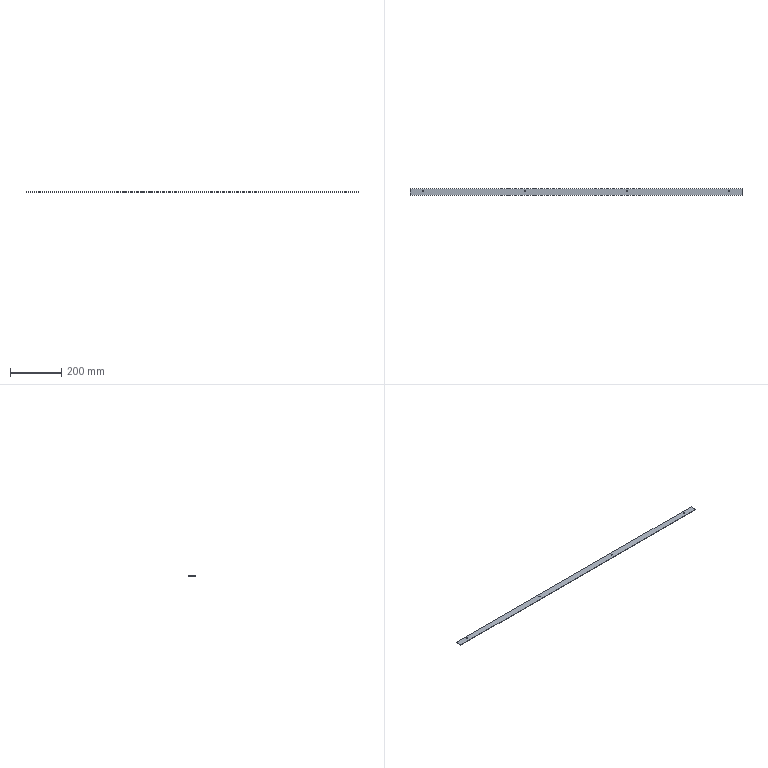Part | STEP file | 1 solid | 14 faces | box 1300 x 25 x 1.5 mm | volume 48655 mm3 | cylinder 8 | plane 6 | commonest cylinder face diameters 4.5 x8
STEP:
#1=CARTESIAN_POINT('',(0.,0.,0.));
#2=DIRECTION('',(0.,0.,1.));
#3=DIRECTION('',(1.,0.,0.));
#4=AXIS2_PLACEMENT_3D('',#1,#2,#3);
#5=CARTESIAN_POINT('',(632.25,-55.,1.5));
#6=VERTEX_POINT('',#5);
#7=CARTESIAN_POINT('',(627.75,-55.,1.5));
#8=VERTEX_POINT('',#7);
#9=CARTESIAN_POINT('',(630.,-55.,1.5));
#10=DIRECTION('',(0.,0.,1.));
#11=DIRECTION('',(1.,0.,0.));
#12=AXIS2_PLACEMENT_3D('',#9,#10,#11);
#13=CIRCLE('',#12,2.25);
#14=CARTESIAN_POINT('',(630.,-55.,1.5));
#15=DIRECTION('',(0.,0.,1.));
#16=DIRECTION('',(1.,0.,0.));
#17=AXIS2_PLACEMENT_3D('',#14,#15,#16);
#18=CYLINDRICAL_SURFACE('',#17,2.25);
#19=CARTESIAN_POINT('',(0.,0.));
#20=DIRECTION('',(1.,0.));
#21=VECTOR('',#20,1.);
#22=LINE('',#19,#21);
#23=(GEOMETRIC_REPRESENTATION_CONTEXT(2)PARAMETRIC_REPRESENTATION_CONTEXT()REPRESENTATION_CONTEXT('',''));
#24=DEFINITIONAL_REPRESENTATION('',(#22),#23);
#25=PCURVE('',#18,#24);
#26=CARTESIAN_POINT('',(0.,0.,1.5));
#27=DIRECTION('',(0.,0.,1.));
#28=DIRECTION('',(1.,0.,0.));
#29=AXIS2_PLACEMENT_3D('',#26,#27,#28);
#30=PLANE('',#29);
#31=CARTESIAN_POINT('',(630.,-55.));
#32=DIRECTION('',(1.,0.));
#33=AXIS2_PLACEMENT_2D('',#31,#32);
#34=CIRCLE('',#33,2.25);
#35=(GEOMETRIC_REPRESENTATION_CONTEXT(2)PARAMETRIC_REPRESENTATION_CONTEXT()REPRESENTATION_CONTEXT('',''));
#36=DEFINITIONAL_REPRESENTATION('',(#34),#35);
#37=PCURVE('',#30,#36);
#38=SURFACE_CURVE('',#13,(#25,#37),.PCURVE_S1.);
#39=EDGE_CURVE('',#6,#8,#38,.T.);
#40=ORIENTED_EDGE('',*,*,#39,.F.);
#41=CARTESIAN_POINT('',(632.25,-55.,0.));
#42=VERTEX_POINT('',#41);
#43=CARTESIAN_POINT('',(632.25,-55.,1.5));
#44=DIRECTION('',(0.,0.,1.));
#45=VECTOR('',#44,1.);
#46=LINE('',#43,#45);
#47=CARTESIAN_POINT('',(0.,0.));
#48=DIRECTION('',(0.,1.));
#49=VECTOR('',#48,1.);
#50=LINE('',#47,#49);
#51=(GEOMETRIC_REPRESENTATION_CONTEXT(2)PARAMETRIC_REPRESENTATION_CONTEXT()REPRESENTATION_CONTEXT('',''));
#52=DEFINITIONAL_REPRESENTATION('',(#50),#51);
#53=PCURVE('',#18,#52);
#54=CARTESIAN_POINT('',(630.,-55.,1.5));
#55=DIRECTION('',(0.,0.,1.));
#56=DIRECTION('',(1.,0.,0.));
#57=AXIS2_PLACEMENT_3D('',#54,#55,#56);
#58=CYLINDRICAL_SURFACE('',#57,2.25);
#59=CARTESIAN_POINT('',(6.283,0.));
#60=DIRECTION('',(0.,1.));
#61=VECTOR('',#60,1.);
#62=LINE('',#59,#61);
#63=(GEOMETRIC_REPRESENTATION_CONTEXT(2)PARAMETRIC_REPRESENTATION_CONTEXT()REPRESENTATION_CONTEXT('',''));
#64=DEFINITIONAL_REPRESENTATION('',(#62),#63);
#65=PCURVE('',#58,#64);
#66=SURFACE_CURVE('',#46,(#53,#65),.PCURVE_S1.);
#67=EDGE_CURVE('',#42,#6,#66,.T.);
#68=ORIENTED_EDGE('',*,*,#67,.F.);
#69=CARTESIAN_POINT('',(627.75,-55.,0.));
#70=VERTEX_POINT('',#69);
#71=CARTESIAN_POINT('',(630.,-55.,0.));
#72=DIRECTION('',(0.,0.,1.));
#73=DIRECTION('',(1.,0.,0.));
#74=AXIS2_PLACEMENT_3D('',#71,#72,#73);
#75=CIRCLE('',#74,2.25);
#76=CARTESIAN_POINT('',(0.,-1.5));
#77=DIRECTION('',(1.,0.));
#78=VECTOR('',#77,1.);
#79=LINE('',#76,#78);
#80=(GEOMETRIC_REPRESENTATION_CONTEXT(2)PARAMETRIC_REPRESENTATION_CONTEXT()REPRESENTATION_CONTEXT('',''));
#81=DEFINITIONAL_REPRESENTATION('',(#79),#80);
#82=PCURVE('',#18,#81);
#83=CARTESIAN_POINT('',(0.,0.,0.));
#84=DIRECTION('',(0.,0.,1.));
#85=DIRECTION('',(1.,0.,0.));
#86=AXIS2_PLACEMENT_3D('',#83,#84,#85);
#87=PLANE('',#86);
#88=CARTESIAN_POINT('',(630.,-55.));
#89=DIRECTION('',(1.,0.));
#90=AXIS2_PLACEMENT_2D('',#88,#89);
#91=CIRCLE('',#90,2.25);
#92=(GEOMETRIC_REPRESENTATION_CONTEXT(2)PARAMETRIC_REPRESENTATION_CONTEXT()REPRESENTATION_CONTEXT('',''));
#93=DEFINITIONAL_REPRESENTATION('',(#91),#92);
#94=PCURVE('',#87,#93);
#95=SURFACE_CURVE('',#75,(#82,#94),.PCURVE_S1.);
#96=EDGE_CURVE('',#42,#70,#95,.T.);
#97=ORIENTED_EDGE('',*,*,#96,.T.);
#98=CARTESIAN_POINT('',(627.75,-55.,1.5));
#99=DIRECTION('',(0.,0.,1.));
#100=VECTOR('',#99,1.);
#101=LINE('',#98,#100);
#102=CARTESIAN_POINT('',(3.142,0.));
#103=DIRECTION('',(0.,1.));
#104=VECTOR('',#103,1.);
#105=LINE('',#102,#104);
#106=(GEOMETRIC_REPRESENTATION_CONTEXT(2)PARAMETRIC_REPRESENTATION_CONTEXT()REPRESENTATION_CONTEXT('',''));
#107=DEFINITIONAL_REPRESENTATION('',(#105),#106);
#108=PCURVE('',#18,#107);
#109=CARTESIAN_POINT('',(3.142,0.));
#110=DIRECTION('',(0.,1.));
#111=VECTOR('',#110,1.);
#112=LINE('',#109,#111);
#113=(GEOMETRIC_REPRESENTATION_CONTEXT(2)PARAMETRIC_REPRESENTATION_CONTEXT()REPRESENTATION_CONTEXT('',''));
#114=DEFINITIONAL_REPRESENTATION('',(#112),#113);
#115=PCURVE('',#58,#114);
#116=SURFACE_CURVE('',#101,(#108,#115),.PCURVE_S1.);
#117=EDGE_CURVE('',#70,#8,#116,.T.);
#118=ORIENTED_EDGE('',*,*,#117,.T.);
#119=EDGE_LOOP('',(#40,#68,#97,#118));
#120=FACE_BOUND('',#119,.F.);
#121=ADVANCED_FACE('',(#120),#18,.F.);
#122=CARTESIAN_POINT('',(1032.25,-55.,1.5));
#123=VERTEX_POINT('',#122);
#124=CARTESIAN_POINT('',(1027.75,-55.,1.5));
#125=VERTEX_POINT('',#124);
#126=CARTESIAN_POINT('',(1030.,-55.,1.5));
#127=DIRECTION('',(0.,0.,1.));
#128=DIRECTION('',(1.,0.,0.));
#129=AXIS2_PLACEMENT_3D('',#126,#127,#128);
#130=CIRCLE('',#129,2.25);
#131=CARTESIAN_POINT('',(1030.,-55.,1.5));
#132=DIRECTION('',(0.,0.,1.));
#133=DIRECTION('',(1.,0.,0.));
#134=AXIS2_PLACEMENT_3D('',#131,#132,#133);
#135=CYLINDRICAL_SURFACE('',#134,2.25);
#136=CARTESIAN_POINT('',(0.,0.));
#137=DIRECTION('',(1.,0.));
#138=VECTOR('',#137,1.);
#139=LINE('',#136,#138);
#140=(GEOMETRIC_REPRESENTATION_CONTEXT(2)PARAMETRIC_REPRESENTATION_CONTEXT()REPRESENTATION_CONTEXT('',''));
#141=DEFINITIONAL_REPRESENTATION('',(#139),#140);
#142=PCURVE('',#135,#141);
#143=CARTESIAN_POINT('',(1030.,-55.));
#144=DIRECTION('',(1.,0.));
#145=AXIS2_PLACEMENT_2D('',#143,#144);
#146=CIRCLE('',#145,2.25);
#147=(GEOMETRIC_REPRESENTATION_CONTEXT(2)PARAMETRIC_REPRESENTATION_CONTEXT()REPRESENTATION_CONTEXT('',''));
#148=DEFINITIONAL_REPRESENTATION('',(#146),#147);
#149=PCURVE('',#30,#148);
#150=SURFACE_CURVE('',#130,(#142,#149),.PCURVE_S1.);
#151=EDGE_CURVE('',#123,#125,#150,.T.);
#152=ORIENTED_EDGE('',*,*,#151,.F.);
#153=CARTESIAN_POINT('',(1032.25,-55.,0.));
#154=VERTEX_POINT('',#153);
#155=CARTESIAN_POINT('',(1032.25,-55.,1.5));
#156=DIRECTION('',(0.,0.,1.));
#157=VECTOR('',#156,1.);
#158=LINE('',#155,#157);
#159=CARTESIAN_POINT('',(0.,0.));
#160=DIRECTION('',(0.,1.));
#161=VECTOR('',#160,1.);
#162=LINE('',#159,#161);
#163=(GEOMETRIC_REPRESENTATION_CONTEXT(2)PARAMETRIC_REPRESENTATION_CONTEXT()REPRESENTATION_CONTEXT('',''));
#164=DEFINITIONAL_REPRESENTATION('',(#162),#163);
#165=PCURVE('',#135,#164);
#166=CARTESIAN_POINT('',(1030.,-55.,1.5));
#167=DIRECTION('',(0.,0.,1.));
#168=DIRECTION('',(1.,0.,0.));
#169=AXIS2_PLACEMENT_3D('',#166,#167,#168);
#170=CYLINDRICAL_SURFACE('',#169,2.25);
#171=CARTESIAN_POINT('',(6.283,0.));
#172=DIRECTION('',(0.,1.));
#173=VECTOR('',#172,1.);
#174=LINE('',#171,#173);
#175=(GEOMETRIC_REPRESENTATION_CONTEXT(2)PARAMETRIC_REPRESENTATION_CONTEXT()REPRESENTATION_CONTEXT('',''));
#176=DEFINITIONAL_REPRESENTATION('',(#174),#175);
#177=PCURVE('',#170,#176);
#178=SURFACE_CURVE('',#158,(#165,#177),.PCURVE_S1.);
#179=EDGE_CURVE('',#154,#123,#178,.T.);
#180=ORIENTED_EDGE('',*,*,#179,.F.);
#181=CARTESIAN_POINT('',(1027.75,-55.,0.));
#182=VERTEX_POINT('',#181);
#183=CARTESIAN_POINT('',(1030.,-55.,0.));
#184=DIRECTION('',(0.,0.,1.));
#185=DIRECTION('',(1.,0.,0.));
#186=AXIS2_PLACEMENT_3D('',#183,#184,#185);
#187=CIRCLE('',#186,2.25);
#188=CARTESIAN_POINT('',(0.,-1.5));
#189=DIRECTION('',(1.,0.));
#190=VECTOR('',#189,1.);
#191=LINE('',#188,#190);
#192=(GEOMETRIC_REPRESENTATION_CONTEXT(2)PARAMETRIC_REPRESENTATION_CONTEXT()REPRESENTATION_CONTEXT('',''));
#193=DEFINITIONAL_REPRESENTATION('',(#191),#192);
#194=PCURVE('',#135,#193);
#195=CARTESIAN_POINT('',(1030.,-55.));
#196=DIRECTION('',(1.,0.));
#197=AXIS2_PLACEMENT_2D('',#195,#196);
#198=CIRCLE('',#197,2.25);
#199=(GEOMETRIC_REPRESENTATION_CONTEXT(2)PARAMETRIC_REPRESENTATION_CONTEXT()REPRESENTATION_CONTEXT('',''));
#200=DEFINITIONAL_REPRESENTATION('',(#198),#199);
#201=PCURVE('',#87,#200);
#202=SURFACE_CURVE('',#187,(#194,#201),.PCURVE_S1.);
#203=EDGE_CURVE('',#154,#182,#202,.T.);
#204=ORIENTED_EDGE('',*,*,#203,.T.);
#205=CARTESIAN_POINT('',(1027.75,-55.,1.5));
#206=DIRECTION('',(0.,0.,1.));
#207=VECTOR('',#206,1.);
#208=LINE('',#205,#207);
#209=CARTESIAN_POINT('',(3.142,0.));
#210=DIRECTION('',(0.,1.));
#211=VECTOR('',#210,1.);
#212=LINE('',#209,#211);
#213=(GEOMETRIC_REPRESENTATION_CONTEXT(2)PARAMETRIC_REPRESENTATION_CONTEXT()REPRESENTATION_CONTEXT('',''));
#214=DEFINITIONAL_REPRESENTATION('',(#212),#213);
#215=PCURVE('',#135,#214);
#216=CARTESIAN_POINT('',(3.142,0.));
#217=DIRECTION('',(0.,1.));
#218=VECTOR('',#217,1.);
#219=LINE('',#216,#218);
#220=(GEOMETRIC_REPRESENTATION_CONTEXT(2)PARAMETRIC_REPRESENTATION_CONTEXT()REPRESENTATION_CONTEXT('',''));
#221=DEFINITIONAL_REPRESENTATION('',(#219),#220);
#222=PCURVE('',#170,#221);
#223=SURFACE_CURVE('',#208,(#215,#222),.PCURVE_S1.);
#224=EDGE_CURVE('',#182,#125,#223,.T.);
#225=ORIENTED_EDGE('',*,*,#224,.T.);
#226=EDGE_LOOP('',(#152,#180,#204,#225));
#227=FACE_BOUND('',#226,.F.);
#228=ADVANCED_FACE('',(#227),#135,.F.);
#229=CARTESIAN_POINT('',(1432.25,-55.,1.5));
#230=VERTEX_POINT('',#229);
#231=CARTESIAN_POINT('',(1427.75,-55.,1.5));
#232=VERTEX_POINT('',#231);
#233=CARTESIAN_POINT('',(1430.,-55.,1.5));
#234=DIRECTION('',(0.,0.,1.));
#235=DIRECTION('',(1.,0.,0.));
#236=AXIS2_PLACEMENT_3D('',#233,#234,#235);
#237=CIRCLE('',#236,2.25);
#238=CARTESIAN_POINT('',(1430.,-55.,1.5));
#239=DIRECTION('',(0.,0.,1.));
#240=DIRECTION('',(1.,0.,0.));
#241=AXIS2_PLACEMENT_3D('',#238,#239,#240);
#242=CYLINDRICAL_SURFACE('',#241,2.25);
#243=CARTESIAN_POINT('',(0.,0.));
#244=DIRECTION('',(1.,0.));
#245=VECTOR('',#244,1.);
#246=LINE('',#243,#245);
#247=(GEOMETRIC_REPRESENTATION_CONTEXT(2)PARAMETRIC_REPRESENTATION_CONTEXT()REPRESENTATION_CONTEXT('',''));
#248=DEFINITIONAL_REPRESENTATION('',(#246),#247);
#249=PCURVE('',#242,#248);
#250=CARTESIAN_POINT('',(1430.,-55.));
#251=DIRECTION('',(1.,0.));
#252=AXIS2_PLACEMENT_2D('',#250,#251);
#253=CIRCLE('',#252,2.25);
#254=(GEOMETRIC_REPRESENTATION_CONTEXT(2)PARAMETRIC_REPRESENTATION_CONTEXT()REPRESENTATION_CONTEXT('',''));
#255=DEFINITIONAL_REPRESENTATION('',(#253),#254);
#256=PCURVE('',#30,#255);
#257=SURFACE_CURVE('',#237,(#249,#256),.PCURVE_S1.);
#258=EDGE_CURVE('',#230,#232,#257,.T.);
#259=ORIENTED_EDGE('',*,*,#258,.F.);
#260=CARTESIAN_POINT('',(1432.25,-55.,0.));
#261=VERTEX_POINT('',#260);
#262=CARTESIAN_POINT('',(1432.25,-55.,1.5));
#263=DIRECTION('',(0.,0.,1.));
#264=VECTOR('',#263,1.);
#265=LINE('',#262,#264);
#266=CARTESIAN_POINT('',(0.,0.));
#267=DIRECTION('',(0.,1.));
#268=VECTOR('',#267,1.);
#269=LINE('',#266,#268);
#270=(GEOMETRIC_REPRESENTATION_CONTEXT(2)PARAMETRIC_REPRESENTATION_CONTEXT()REPRESENTATION_CONTEXT('',''));
#271=DEFINITIONAL_REPRESENTATION('',(#269),#270);
#272=PCURVE('',#242,#271);
#273=CARTESIAN_POINT('',(1430.,-55.,1.5));
#274=DIRECTION('',(0.,0.,1.));
#275=DIRECTION('',(1.,0.,0.));
#276=AXIS2_PLACEMENT_3D('',#273,#274,#275);
#277=CYLINDRICAL_SURFACE('',#276,2.25);
#278=CARTESIAN_POINT('',(6.283,0.));
#279=DIRECTION('',(0.,1.));
#280=VECTOR('',#279,1.);
#281=LINE('',#278,#280);
#282=(GEOMETRIC_REPRESENTATION_CONTEXT(2)PARAMETRIC_REPRESENTATION_CONTEXT()REPRESENTATION_CONTEXT('',''));
#283=DEFINITIONAL_REPRESENTATION('',(#281),#282);
#284=PCURVE('',#277,#283);
#285=SURFACE_CURVE('',#265,(#272,#284),.PCURVE_S1.);
#286=EDGE_CURVE('',#261,#230,#285,.T.);
#287=ORIENTED_EDGE('',*,*,#286,.F.);
#288=CARTESIAN_POINT('',(1427.75,-55.,0.));
#289=VERTEX_POINT('',#288);
#290=CARTESIAN_POINT('',(1430.,-55.,0.));
#291=DIRECTION('',(0.,0.,1.));
#292=DIRECTION('',(1.,0.,0.));
#293=AXIS2_PLACEMENT_3D('',#290,#291,#292);
#294=CIRCLE('',#293,2.25);
#295=CARTESIAN_POINT('',(0.,-1.5));
#296=DIRECTION('',(1.,0.));
#297=VECTOR('',#296,1.);
#298=LINE('',#295,#297);
#299=(GEOMETRIC_REPRESENTATION_CONTEXT(2)PARAMETRIC_REPRESENTATION_CONTEXT()REPRESENTATION_CONTEXT('',''));
#300=DEFINITIONAL_REPRESENTATION('',(#298),#299);
#301=PCURVE('',#242,#300);
#302=CARTESIAN_POINT('',(1430.,-55.));
#303=DIRECTION('',(1.,0.));
#304=AXIS2_PLACEMENT_2D('',#302,#303);
#305=CIRCLE('',#304,2.25);
#306=(GEOMETRIC_REPRESENTATION_CONTEXT(2)PARAMETRIC_REPRESENTATION_CONTEXT()REPRESENTATION_CONTEXT('',''));
#307=DEFINITIONAL_REPRESENTATION('',(#305),#306);
#308=PCURVE('',#87,#307);
#309=SURFACE_CURVE('',#294,(#301,#308),.PCURVE_S1.);
#310=EDGE_CURVE('',#261,#289,#309,.T.);
#311=ORIENTED_EDGE('',*,*,#310,.T.);
#312=CARTESIAN_POINT('',(1427.75,-55.,1.5));
#313=DIRECTION('',(0.,0.,1.));
#314=VECTOR('',#313,1.);
#315=LINE('',#312,#314);
#316=CARTESIAN_POINT('',(3.142,0.));
#317=DIRECTION('',(0.,1.));
#318=VECTOR('',#317,1.);
#319=LINE('',#316,#318);
#320=(GEOMETRIC_REPRESENTATION_CONTEXT(2)PARAMETRIC_REPRESENTATION_CONTEXT()REPRESENTATION_CONTEXT('',''));
#321=DEFINITIONAL_REPRESENTATION('',(#319),#320);
#322=PCURVE('',#242,#321);
#323=CARTESIAN_POINT('',(3.142,0.));
#324=DIRECTION('',(0.,1.));
#325=VECTOR('',#324,1.);
#326=LINE('',#323,#325);
#327=(GEOMETRIC_REPRESENTATION_CONTEXT(2)PARAMETRIC_REPRESENTATION_CONTEXT()REPRESENTATION_CONTEXT('',''));
#328=DEFINITIONAL_REPRESENTATION('',(#326),#327);
#329=PCURVE('',#277,#328);
#330=SURFACE_CURVE('',#315,(#322,#329),.PCURVE_S1.);
#331=EDGE_CURVE('',#289,#232,#330,.T.);
#332=ORIENTED_EDGE('',*,*,#331,.T.);
#333=EDGE_LOOP('',(#259,#287,#311,#332));
#334=FACE_BOUND('',#333,.F.);
#335=ADVANCED_FACE('',(#334),#242,.F.);
#336=CARTESIAN_POINT('',(1832.25,-55.,1.5));
#337=VERTEX_POINT('',#336);
#338=CARTESIAN_POINT('',(1827.75,-55.,1.5));
#339=VERTEX_POINT('',#338);
#340=CARTESIAN_POINT('',(1830.,-55.,1.5));
#341=DIRECTION('',(0.,0.,1.));
#342=DIRECTION('',(1.,0.,0.));
#343=AXIS2_PLACEMENT_3D('',#340,#341,#342);
#344=CIRCLE('',#343,2.25);
#345=CARTESIAN_POINT('',(1830.,-55.,1.5));
#346=DIRECTION('',(0.,0.,1.));
#347=DIRECTION('',(1.,0.,0.));
#348=AXIS2_PLACEMENT_3D('',#345,#346,#347);
#349=CYLINDRICAL_SURFACE('',#348,2.25);
#350=CARTESIAN_POINT('',(0.,0.));
#351=DIRECTION('',(1.,0.));
#352=VECTOR('',#351,1.);
#353=LINE('',#350,#352);
#354=(GEOMETRIC_REPRESENTATION_CONTEXT(2)PARAMETRIC_REPRESENTATION_CONTEXT()REPRESENTATION_CONTEXT('',''));
#355=DEFINITIONAL_REPRESENTATION('',(#353),#354);
#356=PCURVE('',#349,#355);
#357=CARTESIAN_POINT('',(1830.,-55.));
#358=DIRECTION('',(1.,0.));
#359=AXIS2_PLACEMENT_2D('',#357,#358);
#360=CIRCLE('',#359,2.25);
#361=(GEOMETRIC_REPRESENTATION_CONTEXT(2)PARAMETRIC_REPRESENTATION_CONTEXT()REPRESENTATION_CONTEXT('',''));
#362=DEFINITIONAL_REPRESENTATION('',(#360),#361);
#363=PCURVE('',#30,#362);
#364=SURFACE_CURVE('',#344,(#356,#363),.PCURVE_S1.);
#365=EDGE_CURVE('',#337,#339,#364,.T.);
#366=ORIENTED_EDGE('',*,*,#365,.F.);
#367=CARTESIAN_POINT('',(1832.25,-55.,0.));
#368=VERTEX_POINT('',#367);
#369=CARTESIAN_POINT('',(1832.25,-55.,1.5));
#370=DIRECTION('',(0.,0.,1.));
#371=VECTOR('',#370,1.);
#372=LINE('',#369,#371);
#373=CARTESIAN_POINT('',(0.,0.));
#374=DIRECTION('',(0.,1.));
#375=VECTOR('',#374,1.);
#376=LINE('',#373,#375);
#377=(GEOMETRIC_REPRESENTATION_CONTEXT(2)PARAMETRIC_REPRESENTATION_CONTEXT()REPRESENTATION_CONTEXT('',''));
#378=DEFINITIONAL_REPRESENTATION('',(#376),#377);
#379=PCURVE('',#349,#378);
#380=CARTESIAN_POINT('',(1830.,-55.,1.5));
#381=DIRECTION('',(0.,0.,1.));
#382=DIRECTION('',(1.,0.,0.));
#383=AXIS2_PLACEMENT_3D('',#380,#381,#382);
#384=CYLINDRICAL_SURFACE('',#383,2.25);
#385=CARTESIAN_POINT('',(6.283,0.));
#386=DIRECTION('',(0.,1.));
#387=VECTOR('',#386,1.);
#388=LINE('',#385,#387);
#389=(GEOMETRIC_REPRESENTATION_CONTEXT(2)PARAMETRIC_REPRESENTATION_CONTEXT()REPRESENTATION_CONTEXT('',''));
#390=DEFINITIONAL_REPRESENTATION('',(#388),#389);
#391=PCURVE('',#384,#390);
#392=SURFACE_CURVE('',#372,(#379,#391),.PCURVE_S1.);
#393=EDGE_CURVE('',#368,#337,#392,.T.);
#394=ORIENTED_EDGE('',*,*,#393,.F.);
#395=CARTESIAN_POINT('',(1827.75,-55.,0.));
#396=VERTEX_POINT('',#395);
#397=CARTESIAN_POINT('',(1830.,-55.,0.));
#398=DIRECTION('',(0.,0.,1.));
#399=DIRECTION('',(1.,0.,0.));
#400=AXIS2_PLACEMENT_3D('',#397,#398,#399);
#401=CIRCLE('',#400,2.25);
#402=CARTESIAN_POINT('',(0.,-1.5));
#403=DIRECTION('',(1.,0.));
#404=VECTOR('',#403,1.);
#405=LINE('',#402,#404);
#406=(GEOMETRIC_REPRESENTATION_CONTEXT(2)PARAMETRIC_REPRESENTATION_CONTEXT()REPRESENTATION_CONTEXT('',''));
#407=DEFINITIONAL_REPRESENTATION('',(#405),#406);
#408=PCURVE('',#349,#407);
#409=CARTESIAN_POINT('',(1830.,-55.));
#410=DIRECTION('',(1.,0.));
#411=AXIS2_PLACEMENT_2D('',#409,#410);
#412=CIRCLE('',#411,2.25);
#413=(GEOMETRIC_REPRESENTATION_CONTEXT(2)PARAMETRIC_REPRESENTATION_CONTEXT()REPRESENTATION_CONTEXT('',''));
#414=DEFINITIONAL_REPRESENTATION('',(#412),#413);
#415=PCURVE('',#87,#414);
#416=SURFACE_CURVE('',#401,(#408,#415),.PCURVE_S1.);
#417=EDGE_CURVE('',#368,#396,#416,.T.);
#418=ORIENTED_EDGE('',*,*,#417,.T.);
#419=CARTESIAN_POINT('',(1827.75,-55.,1.5));
#420=DIRECTION('',(0.,0.,1.));
#421=VECTOR('',#420,1.);
#422=LINE('',#419,#421);
#423=CARTESIAN_POINT('',(3.142,0.));
#424=DIRECTION('',(0.,1.));
#425=VECTOR('',#424,1.);
#426=LINE('',#423,#425);
#427=(GEOMETRIC_REPRESENTATION_CONTEXT(2)PARAMETRIC_REPRESENTATION_CONTEXT()REPRESENTATION_CONTEXT('',''));
#428=DEFINITIONAL_REPRESENTATION('',(#426),#427);
#429=PCURVE('',#349,#428);
#430=CARTESIAN_POINT('',(3.142,0.));
#431=DIRECTION('',(0.,1.));
#432=VECTOR('',#431,1.);
#433=LINE('',#430,#432);
#434=(GEOMETRIC_REPRESENTATION_CONTEXT(2)PARAMETRIC_REPRESENTATION_CONTEXT()REPRESENTATION_CONTEXT('',''));
#435=DEFINITIONAL_REPRESENTATION('',(#433),#434);
#436=PCURVE('',#384,#435);
#437=SURFACE_CURVE('',#422,(#429,#436),.PCURVE_S1.);
#438=EDGE_CURVE('',#396,#339,#437,.T.);
#439=ORIENTED_EDGE('',*,*,#438,.T.);
#440=EDGE_LOOP('',(#366,#394,#418,#439));
#441=FACE_BOUND('',#440,.F.);
#442=ADVANCED_FACE('',(#441),#349,.F.);
#443=ORIENTED_EDGE('',*,*,#417,.T.);
#444=CARTESIAN_POINT('',(1830.,-55.,0.));
#445=DIRECTION('',(0.,0.,1.));
#446=DIRECTION('',(1.,0.,0.));
#447=AXIS2_PLACEMENT_3D('',#444,#445,#446);
#448=CIRCLE('',#447,2.25);
#449=CARTESIAN_POINT('',(1830.,-55.));
#450=DIRECTION('',(1.,0.));
#451=AXIS2_PLACEMENT_2D('',#449,#450);
#452=CIRCLE('',#451,2.25);
#453=(GEOMETRIC_REPRESENTATION_CONTEXT(2)PARAMETRIC_REPRESENTATION_CONTEXT()REPRESENTATION_CONTEXT('',''));
#454=DEFINITIONAL_REPRESENTATION('',(#452),#453);
#455=PCURVE('',#87,#454);
#456=CARTESIAN_POINT('',(0.,-1.5));
#457=DIRECTION('',(1.,0.));
#458=VECTOR('',#457,1.);
#459=LINE('',#456,#458);
#460=(GEOMETRIC_REPRESENTATION_CONTEXT(2)PARAMETRIC_REPRESENTATION_CONTEXT()REPRESENTATION_CONTEXT('',''));
#461=DEFINITIONAL_REPRESENTATION('',(#459),#460);
#462=PCURVE('',#384,#461);
#463=SURFACE_CURVE('',#448,(#455,#462),.PCURVE_S1.);
#464=EDGE_CURVE('',#396,#368,#463,.T.);
#465=ORIENTED_EDGE('',*,*,#464,.T.);
#466=EDGE_LOOP('',(#443,#465));
#467=FACE_BOUND('',#466,.T.);
#468=ORIENTED_EDGE('',*,*,#310,.T.);
#469=CARTESIAN_POINT('',(1430.,-55.,0.));
#470=DIRECTION('',(0.,0.,1.));
#471=DIRECTION('',(1.,0.,0.));
#472=AXIS2_PLACEMENT_3D('',#469,#470,#471);
#473=CIRCLE('',#472,2.25);
#474=CARTESIAN_POINT('',(1430.,-55.));
#475=DIRECTION('',(1.,0.));
#476=AXIS2_PLACEMENT_2D('',#474,#475);
#477=CIRCLE('',#476,2.25);
#478=(GEOMETRIC_REPRESENTATION_CONTEXT(2)PARAMETRIC_REPRESENTATION_CONTEXT()REPRESENTATION_CONTEXT('',''));
#479=DEFINITIONAL_REPRESENTATION('',(#477),#478);
#480=PCURVE('',#87,#479);
#481=CARTESIAN_POINT('',(0.,-1.5));
#482=DIRECTION('',(1.,0.));
#483=VECTOR('',#482,1.);
#484=LINE('',#481,#483);
#485=(GEOMETRIC_REPRESENTATION_CONTEXT(2)PARAMETRIC_REPRESENTATION_CONTEXT()REPRESENTATION_CONTEXT('',''));
#486=DEFINITIONAL_REPRESENTATION('',(#484),#485);
#487=PCURVE('',#277,#486);
#488=SURFACE_CURVE('',#473,(#480,#487),.PCURVE_S1.);
#489=EDGE_CURVE('',#289,#261,#488,.T.);
#490=ORIENTED_EDGE('',*,*,#489,.T.);
#491=EDGE_LOOP('',(#468,#490));
#492=FACE_BOUND('',#491,.T.);
#493=ORIENTED_EDGE('',*,*,#203,.T.);
#494=CARTESIAN_POINT('',(1030.,-55.,0.));
#495=DIRECTION('',(0.,0.,1.));
#496=DIRECTION('',(1.,0.,0.));
#497=AXIS2_PLACEMENT_3D('',#494,#495,#496);
#498=CIRCLE('',#497,2.25);
#499=CARTESIAN_POINT('',(1030.,-55.));
#500=DIRECTION('',(1.,0.));
#501=AXIS2_PLACEMENT_2D('',#499,#500);
#502=CIRCLE('',#501,2.25);
#503=(GEOMETRIC_REPRESENTATION_CONTEXT(2)PARAMETRIC_REPRESENTATION_CONTEXT()REPRESENTATION_CONTEXT('',''));
#504=DEFINITIONAL_REPRESENTATION('',(#502),#503);
#505=PCURVE('',#87,#504);
#506=CARTESIAN_POINT('',(0.,-1.5));
#507=DIRECTION('',(1.,0.));
#508=VECTOR('',#507,1.);
#509=LINE('',#506,#508);
#510=(GEOMETRIC_REPRESENTATION_CONTEXT(2)PARAMETRIC_REPRESENTATION_CONTEXT()REPRESENTATION_CONTEXT('',''));
#511=DEFINITIONAL_REPRESENTATION('',(#509),#510);
#512=PCURVE('',#170,#511);
#513=SURFACE_CURVE('',#498,(#505,#512),.PCURVE_S1.);
#514=EDGE_CURVE('',#182,#154,#513,.T.);
#515=ORIENTED_EDGE('',*,*,#514,.T.);
#516=EDGE_LOOP('',(#493,#515));
#517=FACE_BOUND('',#516,.T.);
#518=ORIENTED_EDGE('',*,*,#96,.T.);
#519=CARTESIAN_POINT('',(630.,-55.,0.));
#520=DIRECTION('',(0.,0.,1.));
#521=DIRECTION('',(1.,0.,0.));
#522=AXIS2_PLACEMENT_3D('',#519,#520,#521);
#523=CIRCLE('',#522,2.25);
#524=CARTESIAN_POINT('',(630.,-55.));
#525=DIRECTION('',(1.,0.));
#526=AXIS2_PLACEMENT_2D('',#524,#525);
#527=CIRCLE('',#526,2.25);
#528=(GEOMETRIC_REPRESENTATION_CONTEXT(2)PARAMETRIC_REPRESENTATION_CONTEXT()REPRESENTATION_CONTEXT('',''));
#529=DEFINITIONAL_REPRESENTATION('',(#527),#528);
#530=PCURVE('',#87,#529);
#531=CARTESIAN_POINT('',(0.,-1.5));
#532=DIRECTION('',(1.,0.));
#533=VECTOR('',#532,1.);
#534=LINE('',#531,#533);
#535=(GEOMETRIC_REPRESENTATION_CONTEXT(2)PARAMETRIC_REPRESENTATION_CONTEXT()REPRESENTATION_CONTEXT('',''));
#536=DEFINITIONAL_REPRESENTATION('',(#534),#535);
#537=PCURVE('',#58,#536);
#538=SURFACE_CURVE('',#523,(#530,#537),.PCURVE_S1.);
#539=EDGE_CURVE('',#70,#42,#538,.T.);
#540=ORIENTED_EDGE('',*,*,#539,.T.);
#541=EDGE_LOOP('',(#518,#540));
#542=FACE_BOUND('',#541,.T.);
#543=CARTESIAN_POINT('',(1880.,-45.,0.));
#544=VERTEX_POINT('',#543);
#545=CARTESIAN_POINT('',(580.,-45.,0.));
#546=VERTEX_POINT('',#545);
#547=CARTESIAN_POINT('',(1500.,-45.,0.));
#548=DIRECTION('',(-1.,0.,0.));
#549=VECTOR('',#548,1.);
#550=LINE('',#547,#549);
#551=CARTESIAN_POINT('',(1500.,-45.));
#552=DIRECTION('',(-1.,0.));
#553=VECTOR('',#552,1.);
#554=LINE('',#551,#553);
#555=(GEOMETRIC_REPRESENTATION_CONTEXT(2)PARAMETRIC_REPRESENTATION_CONTEXT()REPRESENTATION_CONTEXT('',''));
#556=DEFINITIONAL_REPRESENTATION('',(#554),#555);
#557=PCURVE('',#87,#556);
#558=CARTESIAN_POINT('',(1500.,-45.,1.5));
#559=DIRECTION('',(0.,-1.,0.));
#560=DIRECTION('',(0.,0.,-1.));
#561=AXIS2_PLACEMENT_3D('',#558,#559,#560);
#562=PLANE('',#561);
#563=CARTESIAN_POINT('',(1.5,0.));
#564=DIRECTION('',(0.,-1.));
#565=VECTOR('',#564,1.);
#566=LINE('',#563,#565);
#567=(GEOMETRIC_REPRESENTATION_CONTEXT(2)PARAMETRIC_REPRESENTATION_CONTEXT()REPRESENTATION_CONTEXT('',''));
#568=DEFINITIONAL_REPRESENTATION('',(#566),#567);
#569=PCURVE('',#562,#568);
#570=SURFACE_CURVE('',#550,(#557,#569),.PCURVE_S1.);
#571=EDGE_CURVE('',#544,#546,#570,.T.);
#572=ORIENTED_EDGE('',*,*,#571,.F.);
#573=CARTESIAN_POINT('',(1880.,-70.,0.));
#574=VERTEX_POINT('',#573);
#575=CARTESIAN_POINT('',(1880.,-70.,0.));
#576=DIRECTION('',(0.,1.,0.));
#577=VECTOR('',#576,1.);
#578=LINE('',#575,#577);
#579=CARTESIAN_POINT('',(1880.,-70.));
#580=DIRECTION('',(0.,1.));
#581=VECTOR('',#580,1.);
#582=LINE('',#579,#581);
#583=(GEOMETRIC_REPRESENTATION_CONTEXT(2)PARAMETRIC_REPRESENTATION_CONTEXT()REPRESENTATION_CONTEXT('',''));
#584=DEFINITIONAL_REPRESENTATION('',(#582),#583);
#585=PCURVE('',#87,#584);
#586=CARTESIAN_POINT('',(1880.,-70.,1.5));
#587=DIRECTION('',(-1.,0.,0.));
#588=DIRECTION('',(0.,0.,1.));
#589=AXIS2_PLACEMENT_3D('',#586,#587,#588);
#590=PLANE('',#589);
#591=CARTESIAN_POINT('',(-1.5,0.));
#592=DIRECTION('',(0.,1.));
#593=VECTOR('',#592,1.);
#594=LINE('',#591,#593);
#595=(GEOMETRIC_REPRESENTATION_CONTEXT(2)PARAMETRIC_REPRESENTATION_CONTEXT()REPRESENTATION_CONTEXT('',''));
#596=DEFINITIONAL_REPRESENTATION('',(#594),#595);
#597=PCURVE('',#590,#596);
#598=SURFACE_CURVE('',#578,(#585,#597),.PCURVE_S1.);
#599=EDGE_CURVE('',#574,#544,#598,.T.);
#600=ORIENTED_EDGE('',*,*,#599,.F.);
#601=CARTESIAN_POINT('',(580.,-70.,0.));
#602=VERTEX_POINT('',#601);
#603=CARTESIAN_POINT('',(600.,-70.,0.));
#604=DIRECTION('',(1.,0.,0.));
#605=VECTOR('',#604,1.);
#606=LINE('',#603,#605);
#607=CARTESIAN_POINT('',(600.,-70.));
#608=DIRECTION('',(1.,0.));
#609=VECTOR('',#608,1.);
#610=LINE('',#607,#609);
#611=(GEOMETRIC_REPRESENTATION_CONTEXT(2)PARAMETRIC_REPRESENTATION_CONTEXT()REPRESENTATION_CONTEXT('',''));
#612=DEFINITIONAL_REPRESENTATION('',(#610),#611);
#613=PCURVE('',#87,#612);
#614=CARTESIAN_POINT('',(600.,-70.,1.5));
#615=DIRECTION('',(0.,1.,0.));
#616=DIRECTION('',(1.,0.,0.));
#617=AXIS2_PLACEMENT_3D('',#614,#615,#616);
#618=PLANE('',#617);
#619=CARTESIAN_POINT('',(0.,1.5));
#620=DIRECTION('',(1.,0.));
#621=VECTOR('',#620,1.);
#622=LINE('',#619,#621);
#623=(GEOMETRIC_REPRESENTATION_CONTEXT(2)PARAMETRIC_REPRESENTATION_CONTEXT()REPRESENTATION_CONTEXT('',''));
#624=DEFINITIONAL_REPRESENTATION('',(#622),#623);
#625=PCURVE('',#618,#624);
#626=SURFACE_CURVE('',#606,(#613,#625),.PCURVE_S1.);
#627=EDGE_CURVE('',#602,#574,#626,.T.);
#628=ORIENTED_EDGE('',*,*,#627,.F.);
#629=CARTESIAN_POINT('',(580.,-45.,0.));
#630=DIRECTION('',(0.,-1.,0.));
#631=VECTOR('',#630,1.);
#632=LINE('',#629,#631);
#633=CARTESIAN_POINT('',(580.,-45.));
#634=DIRECTION('',(0.,-1.));
#635=VECTOR('',#634,1.);
#636=LINE('',#633,#635);
#637=(GEOMETRIC_REPRESENTATION_CONTEXT(2)PARAMETRIC_REPRESENTATION_CONTEXT()REPRESENTATION_CONTEXT('',''));
#638=DEFINITIONAL_REPRESENTATION('',(#636),#637);
#639=PCURVE('',#87,#638);
#640=CARTESIAN_POINT('',(580.,-45.,1.5));
#641=DIRECTION('',(1.,0.,0.));
#642=DIRECTION('',(0.,1.,0.));
#643=AXIS2_PLACEMENT_3D('',#640,#641,#642);
#644=PLANE('',#643);
#645=CARTESIAN_POINT('',(0.,-1.5));
#646=DIRECTION('',(-1.,0.));
#647=VECTOR('',#646,1.);
#648=LINE('',#645,#647);
#649=(GEOMETRIC_REPRESENTATION_CONTEXT(2)PARAMETRIC_REPRESENTATION_CONTEXT()REPRESENTATION_CONTEXT('',''));
#650=DEFINITIONAL_REPRESENTATION('',(#648),#649);
#651=PCURVE('',#644,#650);
#652=SURFACE_CURVE('',#632,(#639,#651),.PCURVE_S1.);
#653=EDGE_CURVE('',#546,#602,#652,.T.);
#654=ORIENTED_EDGE('',*,*,#653,.F.);
#655=EDGE_LOOP('',(#572,#600,#628,#654));
#656=FACE_BOUND('',#655,.T.);
#657=ADVANCED_FACE('',(#467,#492,#517,#542,#656),#87,.F.);
#658=ORIENTED_EDGE('',*,*,#365,.F.);
#659=CARTESIAN_POINT('',(1830.,-55.,1.5));
#660=DIRECTION('',(0.,0.,1.));
#661=DIRECTION('',(1.,0.,0.));
#662=AXIS2_PLACEMENT_3D('',#659,#660,#661);
#663=CIRCLE('',#662,2.25);
#664=CARTESIAN_POINT('',(1830.,-55.));
#665=DIRECTION('',(1.,0.));
#666=AXIS2_PLACEMENT_2D('',#664,#665);
#667=CIRCLE('',#666,2.25);
#668=(GEOMETRIC_REPRESENTATION_CONTEXT(2)PARAMETRIC_REPRESENTATION_CONTEXT()REPRESENTATION_CONTEXT('',''));
#669=DEFINITIONAL_REPRESENTATION('',(#667),#668);
#670=PCURVE('',#30,#669);
#671=CARTESIAN_POINT('',(0.,0.));
#672=DIRECTION('',(1.,0.));
#673=VECTOR('',#672,1.);
#674=LINE('',#671,#673);
#675=(GEOMETRIC_REPRESENTATION_CONTEXT(2)PARAMETRIC_REPRESENTATION_CONTEXT()REPRESENTATION_CONTEXT('',''));
#676=DEFINITIONAL_REPRESENTATION('',(#674),#675);
#677=PCURVE('',#384,#676);
#678=SURFACE_CURVE('',#663,(#670,#677),.PCURVE_S1.);
#679=EDGE_CURVE('',#339,#337,#678,.T.);
#680=ORIENTED_EDGE('',*,*,#679,.F.);
#681=EDGE_LOOP('',(#658,#680));
#682=FACE_BOUND('',#681,.T.);
#683=ORIENTED_EDGE('',*,*,#258,.F.);
#684=CARTESIAN_POINT('',(1430.,-55.,1.5));
#685=DIRECTION('',(0.,0.,1.));
#686=DIRECTION('',(1.,0.,0.));
#687=AXIS2_PLACEMENT_3D('',#684,#685,#686);
#688=CIRCLE('',#687,2.25);
#689=CARTESIAN_POINT('',(1430.,-55.));
#690=DIRECTION('',(1.,0.));
#691=AXIS2_PLACEMENT_2D('',#689,#690);
#692=CIRCLE('',#691,2.25);
#693=(GEOMETRIC_REPRESENTATION_CONTEXT(2)PARAMETRIC_REPRESENTATION_CONTEXT()REPRESENTATION_CONTEXT('',''));
#694=DEFINITIONAL_REPRESENTATION('',(#692),#693);
#695=PCURVE('',#30,#694);
#696=CARTESIAN_POINT('',(0.,0.));
#697=DIRECTION('',(1.,0.));
#698=VECTOR('',#697,1.);
#699=LINE('',#696,#698);
#700=(GEOMETRIC_REPRESENTATION_CONTEXT(2)PARAMETRIC_REPRESENTATION_CONTEXT()REPRESENTATION_CONTEXT('',''));
#701=DEFINITIONAL_REPRESENTATION('',(#699),#700);
#702=PCURVE('',#277,#701);
#703=SURFACE_CURVE('',#688,(#695,#702),.PCURVE_S1.);
#704=EDGE_CURVE('',#232,#230,#703,.T.);
#705=ORIENTED_EDGE('',*,*,#704,.F.);
#706=EDGE_LOOP('',(#683,#705));
#707=FACE_BOUND('',#706,.T.);
#708=ORIENTED_EDGE('',*,*,#151,.F.);
#709=CARTESIAN_POINT('',(1030.,-55.,1.5));
#710=DIRECTION('',(0.,0.,1.));
#711=DIRECTION('',(1.,0.,0.));
#712=AXIS2_PLACEMENT_3D('',#709,#710,#711);
#713=CIRCLE('',#712,2.25);
#714=CARTESIAN_POINT('',(1030.,-55.));
#715=DIRECTION('',(1.,0.));
#716=AXIS2_PLACEMENT_2D('',#714,#715);
#717=CIRCLE('',#716,2.25);
#718=(GEOMETRIC_REPRESENTATION_CONTEXT(2)PARAMETRIC_REPRESENTATION_CONTEXT()REPRESENTATION_CONTEXT('',''));
#719=DEFINITIONAL_REPRESENTATION('',(#717),#718);
#720=PCURVE('',#30,#719);
#721=CARTESIAN_POINT('',(0.,0.));
#722=DIRECTION('',(1.,0.));
#723=VECTOR('',#722,1.);
#724=LINE('',#721,#723);
#725=(GEOMETRIC_REPRESENTATION_CONTEXT(2)PARAMETRIC_REPRESENTATION_CONTEXT()REPRESENTATION_CONTEXT('',''));
#726=DEFINITIONAL_REPRESENTATION('',(#724),#725);
#727=PCURVE('',#170,#726);
#728=SURFACE_CURVE('',#713,(#720,#727),.PCURVE_S1.);
#729=EDGE_CURVE('',#125,#123,#728,.T.);
#730=ORIENTED_EDGE('',*,*,#729,.F.);
#731=EDGE_LOOP('',(#708,#730));
#732=FACE_BOUND('',#731,.T.);
#733=ORIENTED_EDGE('',*,*,#39,.F.);
#734=CARTESIAN_POINT('',(630.,-55.,1.5));
#735=DIRECTION('',(0.,0.,1.));
#736=DIRECTION('',(1.,0.,0.));
#737=AXIS2_PLACEMENT_3D('',#734,#735,#736);
#738=CIRCLE('',#737,2.25);
#739=CARTESIAN_POINT('',(630.,-55.));
#740=DIRECTION('',(1.,0.));
#741=AXIS2_PLACEMENT_2D('',#739,#740);
#742=CIRCLE('',#741,2.25);
#743=(GEOMETRIC_REPRESENTATION_CONTEXT(2)PARAMETRIC_REPRESENTATION_CONTEXT()REPRESENTATION_CONTEXT('',''));
#744=DEFINITIONAL_REPRESENTATION('',(#742),#743);
#745=PCURVE('',#30,#744);
#746=CARTESIAN_POINT('',(0.,0.));
#747=DIRECTION('',(1.,0.));
#748=VECTOR('',#747,1.);
#749=LINE('',#746,#748);
#750=(GEOMETRIC_REPRESENTATION_CONTEXT(2)PARAMETRIC_REPRESENTATION_CONTEXT()REPRESENTATION_CONTEXT('',''));
#751=DEFINITIONAL_REPRESENTATION('',(#749),#750);
#752=PCURVE('',#58,#751);
#753=SURFACE_CURVE('',#738,(#745,#752),.PCURVE_S1.);
#754=EDGE_CURVE('',#8,#6,#753,.T.);
#755=ORIENTED_EDGE('',*,*,#754,.F.);
#756=EDGE_LOOP('',(#733,#755));
#757=FACE_BOUND('',#756,.T.);
#758=CARTESIAN_POINT('',(1880.,-45.,1.5));
#759=VERTEX_POINT('',#758);
#760=CARTESIAN_POINT('',(580.,-45.,1.5));
#761=VERTEX_POINT('',#760);
#762=CARTESIAN_POINT('',(1500.,-45.,1.5));
#763=DIRECTION('',(-1.,0.,0.));
#764=VECTOR('',#763,1.);
#765=LINE('',#762,#764);
#766=CARTESIAN_POINT('',(1500.,-45.));
#767=DIRECTION('',(-1.,0.));
#768=VECTOR('',#767,1.);
#769=LINE('',#766,#768);
#770=(GEOMETRIC_REPRESENTATION_CONTEXT(2)PARAMETRIC_REPRESENTATION_CONTEXT()REPRESENTATION_CONTEXT('',''));
#771=DEFINITIONAL_REPRESENTATION('',(#769),#770);
#772=PCURVE('',#30,#771);
#773=CARTESIAN_POINT('',(0.,0.));
#774=DIRECTION('',(0.,-1.));
#775=VECTOR('',#774,1.);
#776=LINE('',#773,#775);
#777=(GEOMETRIC_REPRESENTATION_CONTEXT(2)PARAMETRIC_REPRESENTATION_CONTEXT()REPRESENTATION_CONTEXT('',''));
#778=DEFINITIONAL_REPRESENTATION('',(#776),#777);
#779=PCURVE('',#562,#778);
#780=SURFACE_CURVE('',#765,(#772,#779),.PCURVE_S1.);
#781=EDGE_CURVE('',#759,#761,#780,.T.);
#782=ORIENTED_EDGE('',*,*,#781,.T.);
#783=CARTESIAN_POINT('',(580.,-70.,1.5));
#784=VERTEX_POINT('',#783);
#785=CARTESIAN_POINT('',(580.,-45.,1.5));
#786=DIRECTION('',(0.,-1.,0.));
#787=VECTOR('',#786,1.);
#788=LINE('',#785,#787);
#789=CARTESIAN_POINT('',(580.,-45.));
#790=DIRECTION('',(0.,-1.));
#791=VECTOR('',#790,1.);
#792=LINE('',#789,#791);
#793=(GEOMETRIC_REPRESENTATION_CONTEXT(2)PARAMETRIC_REPRESENTATION_CONTEXT()REPRESENTATION_CONTEXT('',''));
#794=DEFINITIONAL_REPRESENTATION('',(#792),#793);
#795=PCURVE('',#30,#794);
#796=CARTESIAN_POINT('',(0.,0.));
#797=DIRECTION('',(-1.,0.));
#798=VECTOR('',#797,1.);
#799=LINE('',#796,#798);
#800=(GEOMETRIC_REPRESENTATION_CONTEXT(2)PARAMETRIC_REPRESENTATION_CONTEXT()REPRESENTATION_CONTEXT('',''));
#801=DEFINITIONAL_REPRESENTATION('',(#799),#800);
#802=PCURVE('',#644,#801);
#803=SURFACE_CURVE('',#788,(#795,#802),.PCURVE_S1.);
#804=EDGE_CURVE('',#761,#784,#803,.T.);
#805=ORIENTED_EDGE('',*,*,#804,.T.);
#806=CARTESIAN_POINT('',(1880.,-70.,1.5));
#807=VERTEX_POINT('',#806);
#808=CARTESIAN_POINT('',(600.,-70.,1.5));
#809=DIRECTION('',(1.,0.,0.));
#810=VECTOR('',#809,1.);
#811=LINE('',#808,#810);
#812=CARTESIAN_POINT('',(600.,-70.));
#813=DIRECTION('',(1.,0.));
#814=VECTOR('',#813,1.);
#815=LINE('',#812,#814);
#816=(GEOMETRIC_REPRESENTATION_CONTEXT(2)PARAMETRIC_REPRESENTATION_CONTEXT()REPRESENTATION_CONTEXT('',''));
#817=DEFINITIONAL_REPRESENTATION('',(#815),#816);
#818=PCURVE('',#30,#817);
#819=CARTESIAN_POINT('',(0.,0.));
#820=DIRECTION('',(1.,0.));
#821=VECTOR('',#820,1.);
#822=LINE('',#819,#821);
#823=(GEOMETRIC_REPRESENTATION_CONTEXT(2)PARAMETRIC_REPRESENTATION_CONTEXT()REPRESENTATION_CONTEXT('',''));
#824=DEFINITIONAL_REPRESENTATION('',(#822),#823);
#825=PCURVE('',#618,#824);
#826=SURFACE_CURVE('',#811,(#818,#825),.PCURVE_S1.);
#827=EDGE_CURVE('',#784,#807,#826,.T.);
#828=ORIENTED_EDGE('',*,*,#827,.T.);
#829=CARTESIAN_POINT('',(1880.,-70.,1.5));
#830=DIRECTION('',(0.,1.,0.));
#831=VECTOR('',#830,1.);
#832=LINE('',#829,#831);
#833=CARTESIAN_POINT('',(1880.,-70.));
#834=DIRECTION('',(0.,1.));
#835=VECTOR('',#834,1.);
#836=LINE('',#833,#835);
#837=(GEOMETRIC_REPRESENTATION_CONTEXT(2)PARAMETRIC_REPRESENTATION_CONTEXT()REPRESENTATION_CONTEXT('',''));
#838=DEFINITIONAL_REPRESENTATION('',(#836),#837);
#839=PCURVE('',#30,#838);
#840=CARTESIAN_POINT('',(0.,0.));
#841=DIRECTION('',(0.,1.));
#842=VECTOR('',#841,1.);
#843=LINE('',#840,#842);
#844=(GEOMETRIC_REPRESENTATION_CONTEXT(2)PARAMETRIC_REPRESENTATION_CONTEXT()REPRESENTATION_CONTEXT('',''));
#845=DEFINITIONAL_REPRESENTATION('',(#843),#844);
#846=PCURVE('',#590,#845);
#847=SURFACE_CURVE('',#832,(#839,#846),.PCURVE_S1.);
#848=EDGE_CURVE('',#807,#759,#847,.T.);
#849=ORIENTED_EDGE('',*,*,#848,.T.);
#850=EDGE_LOOP('',(#782,#805,#828,#849));
#851=FACE_BOUND('',#850,.T.);
#852=ADVANCED_FACE('',(#682,#707,#732,#757,#851),#30,.T.);
#853=ORIENTED_EDGE('',*,*,#599,.T.);
#854=CARTESIAN_POINT('',(1880.,-45.,1.5));
#855=DIRECTION('',(0.,0.,-1.));
#856=VECTOR('',#855,1.);
#857=LINE('',#854,#856);
#858=CARTESIAN_POINT('',(0.,25.));
#859=DIRECTION('',(-1.,0.));
#860=VECTOR('',#859,1.);
#861=LINE('',#858,#860);
#862=(GEOMETRIC_REPRESENTATION_CONTEXT(2)PARAMETRIC_REPRESENTATION_CONTEXT()REPRESENTATION_CONTEXT('',''));
#863=DEFINITIONAL_REPRESENTATION('',(#861),#862);
#864=PCURVE('',#590,#863);
#865=CARTESIAN_POINT('',(0.,380.));
#866=DIRECTION('',(1.,0.));
#867=VECTOR('',#866,1.);
#868=LINE('',#865,#867);
#869=(GEOMETRIC_REPRESENTATION_CONTEXT(2)PARAMETRIC_REPRESENTATION_CONTEXT()REPRESENTATION_CONTEXT('',''));
#870=DEFINITIONAL_REPRESENTATION('',(#868),#869);
#871=PCURVE('',#562,#870);
#872=SURFACE_CURVE('',#857,(#864,#871),.PCURVE_S1.);
#873=EDGE_CURVE('',#759,#544,#872,.T.);
#874=ORIENTED_EDGE('',*,*,#873,.F.);
#875=ORIENTED_EDGE('',*,*,#848,.F.);
#876=CARTESIAN_POINT('',(1880.,-70.,1.5));
#877=DIRECTION('',(0.,0.,-1.));
#878=VECTOR('',#877,1.);
#879=LINE('',#876,#878);
#880=CARTESIAN_POINT('',(0.,0.));
#881=DIRECTION('',(-1.,0.));
#882=VECTOR('',#881,1.);
#883=LINE('',#880,#882);
#884=(GEOMETRIC_REPRESENTATION_CONTEXT(2)PARAMETRIC_REPRESENTATION_CONTEXT()REPRESENTATION_CONTEXT('',''));
#885=DEFINITIONAL_REPRESENTATION('',(#883),#884);
#886=PCURVE('',#590,#885);
#887=CARTESIAN_POINT('',(1280.,0.));
#888=DIRECTION('',(0.,1.));
#889=VECTOR('',#888,1.);
#890=LINE('',#887,#889);
#891=(GEOMETRIC_REPRESENTATION_CONTEXT(2)PARAMETRIC_REPRESENTATION_CONTEXT()REPRESENTATION_CONTEXT('',''));
#892=DEFINITIONAL_REPRESENTATION('',(#890),#891);
#893=PCURVE('',#618,#892);
#894=SURFACE_CURVE('',#879,(#886,#893),.PCURVE_S1.);
#895=EDGE_CURVE('',#807,#574,#894,.T.);
#896=ORIENTED_EDGE('',*,*,#895,.T.);
#897=EDGE_LOOP('',(#853,#874,#875,#896));
#898=FACE_BOUND('',#897,.T.);
#899=ADVANCED_FACE('',(#898),#590,.F.);
#900=ORIENTED_EDGE('',*,*,#627,.T.);
#901=ORIENTED_EDGE('',*,*,#895,.F.);
#902=ORIENTED_EDGE('',*,*,#827,.F.);
#903=CARTESIAN_POINT('',(580.,-70.,1.5));
#904=DIRECTION('',(0.,0.,-1.));
#905=VECTOR('',#904,1.);
#906=LINE('',#903,#905);
#907=CARTESIAN_POINT('',(-20.,0.));
#908=DIRECTION('',(0.,1.));
#909=VECTOR('',#908,1.);
#910=LINE('',#907,#909);
#911=(GEOMETRIC_REPRESENTATION_CONTEXT(2)PARAMETRIC_REPRESENTATION_CONTEXT()REPRESENTATION_CONTEXT('',''));
#912=DEFINITIONAL_REPRESENTATION('',(#910),#911);
#913=PCURVE('',#618,#912);
#914=CARTESIAN_POINT('',(-25.,0.));
#915=DIRECTION('',(0.,-1.));
#916=VECTOR('',#915,1.);
#917=LINE('',#914,#916);
#918=(GEOMETRIC_REPRESENTATION_CONTEXT(2)PARAMETRIC_REPRESENTATION_CONTEXT()REPRESENTATION_CONTEXT('',''));
#919=DEFINITIONAL_REPRESENTATION('',(#917),#918);
#920=PCURVE('',#644,#919);
#921=SURFACE_CURVE('',#906,(#913,#920),.PCURVE_S1.);
#922=EDGE_CURVE('',#784,#602,#921,.T.);
#923=ORIENTED_EDGE('',*,*,#922,.T.);
#924=EDGE_LOOP('',(#900,#901,#902,#923));
#925=FACE_BOUND('',#924,.T.);
#926=ADVANCED_FACE('',(#925),#618,.F.);
#927=ORIENTED_EDGE('',*,*,#653,.T.);
#928=ORIENTED_EDGE('',*,*,#922,.F.);
#929=ORIENTED_EDGE('',*,*,#804,.F.);
#930=CARTESIAN_POINT('',(580.,-45.,1.5));
#931=DIRECTION('',(0.,0.,-1.));
#932=VECTOR('',#931,1.);
#933=LINE('',#930,#932);
#934=CARTESIAN_POINT('',(0.,0.));
#935=DIRECTION('',(0.,-1.));
#936=VECTOR('',#935,1.);
#937=LINE('',#934,#936);
#938=(GEOMETRIC_REPRESENTATION_CONTEXT(2)PARAMETRIC_REPRESENTATION_CONTEXT()REPRESENTATION_CONTEXT('',''));
#939=DEFINITIONAL_REPRESENTATION('',(#937),#938);
#940=PCURVE('',#644,#939);
#941=CARTESIAN_POINT('',(0.,-920.));
#942=DIRECTION('',(1.,0.));
#943=VECTOR('',#942,1.);
#944=LINE('',#941,#943);
#945=(GEOMETRIC_REPRESENTATION_CONTEXT(2)PARAMETRIC_REPRESENTATION_CONTEXT()REPRESENTATION_CONTEXT('',''));
#946=DEFINITIONAL_REPRESENTATION('',(#944),#945);
#947=PCURVE('',#562,#946);
#948=SURFACE_CURVE('',#933,(#940,#947),.PCURVE_S1.);
#949=EDGE_CURVE('',#761,#546,#948,.T.);
#950=ORIENTED_EDGE('',*,*,#949,.T.);
#951=EDGE_LOOP('',(#927,#928,#929,#950));
#952=FACE_BOUND('',#951,.T.);
#953=ADVANCED_FACE('',(#952),#644,.F.);
#954=ORIENTED_EDGE('',*,*,#571,.T.);
#955=ORIENTED_EDGE('',*,*,#949,.F.);
#956=ORIENTED_EDGE('',*,*,#781,.F.);
#957=ORIENTED_EDGE('',*,*,#873,.T.);
#958=EDGE_LOOP('',(#954,#955,#956,#957));
#959=FACE_BOUND('',#958,.T.);
#960=ADVANCED_FACE('',(#959),#562,.F.);
#961=ORIENTED_EDGE('',*,*,#393,.T.);
#962=ORIENTED_EDGE('',*,*,#679,.F.);
#963=ORIENTED_EDGE('',*,*,#438,.F.);
#964=ORIENTED_EDGE('',*,*,#464,.T.);
#965=EDGE_LOOP('',(#961,#962,#963,#964));
#966=FACE_BOUND('',#965,.F.);
#967=ADVANCED_FACE('',(#966),#384,.F.);
#968=ORIENTED_EDGE('',*,*,#286,.T.);
#969=ORIENTED_EDGE('',*,*,#704,.F.);
#970=ORIENTED_EDGE('',*,*,#331,.F.);
#971=ORIENTED_EDGE('',*,*,#489,.T.);
#972=EDGE_LOOP('',(#968,#969,#970,#971));
#973=FACE_BOUND('',#972,.F.);
#974=ADVANCED_FACE('',(#973),#277,.F.);
#975=ORIENTED_EDGE('',*,*,#179,.T.);
#976=ORIENTED_EDGE('',*,*,#729,.F.);
#977=ORIENTED_EDGE('',*,*,#224,.F.);
#978=ORIENTED_EDGE('',*,*,#514,.T.);
#979=EDGE_LOOP('',(#975,#976,#977,#978));
#980=FACE_BOUND('',#979,.F.);
#981=ADVANCED_FACE('',(#980),#170,.F.);
#982=ORIENTED_EDGE('',*,*,#67,.T.);
#983=ORIENTED_EDGE('',*,*,#754,.F.);
#984=ORIENTED_EDGE('',*,*,#117,.F.);
#985=ORIENTED_EDGE('',*,*,#539,.T.);
#986=EDGE_LOOP('',(#982,#983,#984,#985));
#987=FACE_BOUND('',#986,.F.);
#988=ADVANCED_FACE('',(#987),#58,.F.);
#989=CLOSED_SHELL('',(#121,#228,#335,#442,#657,#852,#899,#926,#953,#960,#967,#974,#981,#988));
#990=MANIFOLD_SOLID_BREP('',#989);
#991=(LENGTH_UNIT()NAMED_UNIT(*)SI_UNIT(.MILLI.,.METRE.));
#992=UNCERTAINTY_MEASURE_WITH_UNIT(LENGTH_MEASURE(0.0000001),#991,'','');
#993=(NAMED_UNIT(*)PLANE_ANGLE_UNIT()SI_UNIT($,.RADIAN.));
#994=(NAMED_UNIT(*)SI_UNIT($,.STERADIAN.)SOLID_ANGLE_UNIT());
#995=(GEOMETRIC_REPRESENTATION_CONTEXT(3)GLOBAL_UNCERTAINTY_ASSIGNED_CONTEXT((#992))GLOBAL_UNIT_ASSIGNED_CONTEXT((#991,#993,#994))REPRESENTATION_CONTEXT('',''));
#996=ADVANCED_BREP_SHAPE_REPRESENTATION('',(#4,#990),#995);